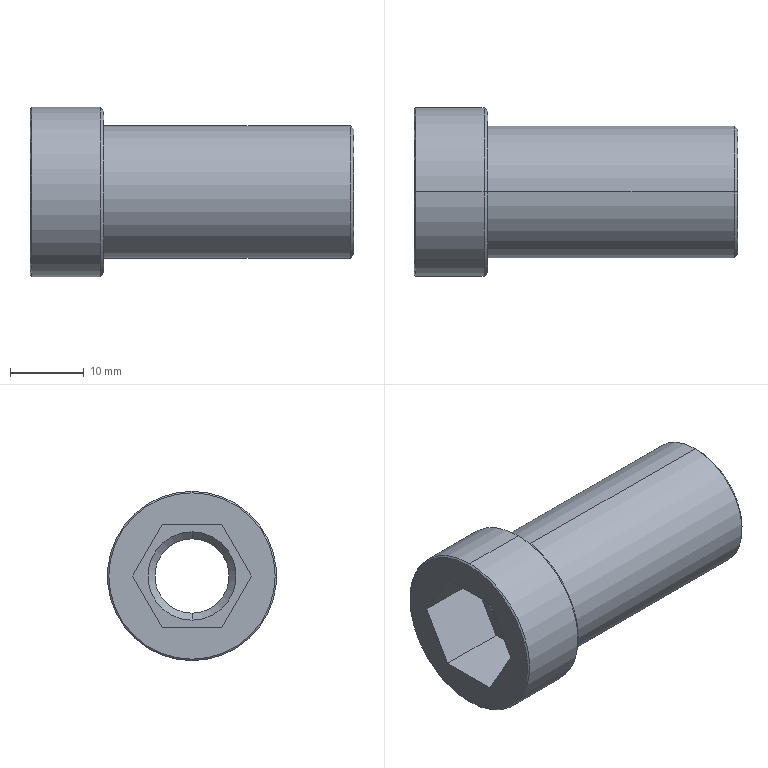Part | STEP file | SI125 | 1 solid | 26 faces | box 44 x 23 x 23 mm | volume 8397 mm3 | cone 10 | plane 10 | cylinder 6 | commonest cylinder face diameters 10.106 x2 18 x2 23 x2